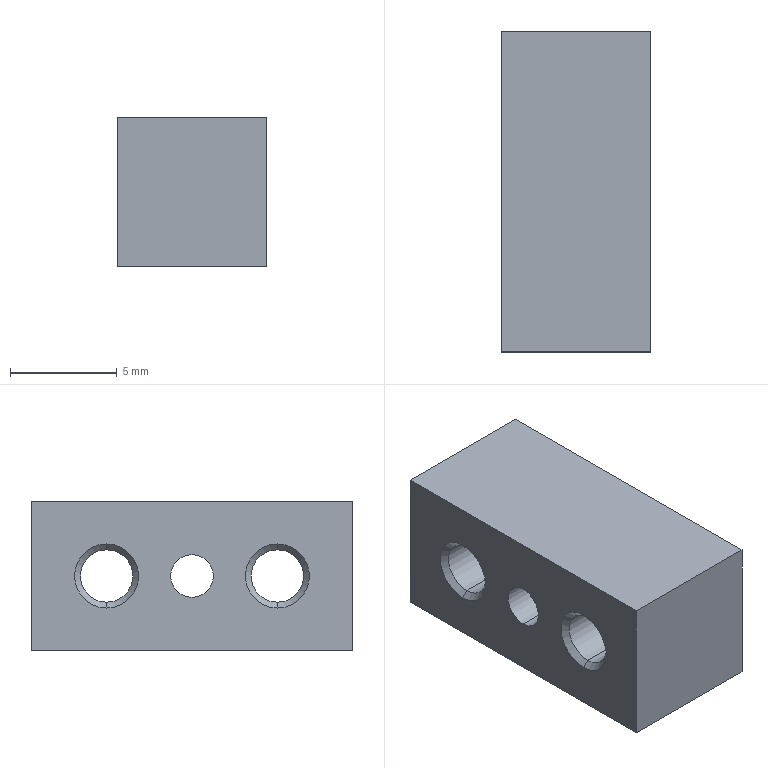Part | STEP file | 1 solid | 20 faces | box 7 x 15 x 7 mm | volume 645.309 mm3 | cone 8 | cylinder 6 | plane 6 | commonest cylinder face diameters 2.459 x4 2 x2
STEP:
#1=CARTESIAN_POINT('',(0.,0.,0.));
#2=DIRECTION('',(0.,0.,1.));
#3=DIRECTION('',(1.,0.,0.));
#4=AXIS2_PLACEMENT_3D('',#1,#2,#3);
#5=CARTESIAN_POINT('',(6.729,11.5,-1.23));
#6=VERTEX_POINT('',#5);
#7=CARTESIAN_POINT('',(7.,11.5,-1.5));
#8=VERTEX_POINT('',#7);
#9=CARTESIAN_POINT('',(7.,11.5,-1.5));
#10=DIRECTION('',(0.7071,0.,-0.7071));
#11=VECTOR('',#10,1.);
#12=LINE('',#9,#11);
#13=CARTESIAN_POINT('',(7.,11.5,0.));
#14=DIRECTION('',(1.,0.,0.));
#15=DIRECTION('',(0.,0.,-1.));
#16=AXIS2_PLACEMENT_3D('',#13,#14,#15);
#17=CONICAL_SURFACE('',#16,1.5,0.7854);
#18=CARTESIAN_POINT('',(6.283,0.));
#19=DIRECTION('',(0.,1.));
#20=VECTOR('',#19,1.);
#21=LINE('',#18,#20);
#22=(GEOMETRIC_REPRESENTATION_CONTEXT(2)PARAMETRIC_REPRESENTATION_CONTEXT()REPRESENTATION_CONTEXT('',''));
#23=DEFINITIONAL_REPRESENTATION('',(#21),#22);
#24=PCURVE('',#17,#23);
#25=CARTESIAN_POINT('',(7.,11.5,0.));
#26=DIRECTION('',(1.,0.,0.));
#27=DIRECTION('',(0.,0.,-1.));
#28=AXIS2_PLACEMENT_3D('',#25,#26,#27);
#29=CONICAL_SURFACE('',#28,1.5,0.7854);
#30=CARTESIAN_POINT('',(0.,0.));
#31=DIRECTION('',(0.,1.));
#32=VECTOR('',#31,1.);
#33=LINE('',#30,#32);
#34=(GEOMETRIC_REPRESENTATION_CONTEXT(2)PARAMETRIC_REPRESENTATION_CONTEXT()REPRESENTATION_CONTEXT('',''));
#35=DEFINITIONAL_REPRESENTATION('',(#33),#34);
#36=PCURVE('',#29,#35);
#37=SURFACE_CURVE('',#12,(#24,#36),.PCURVE_S1.);
#38=EDGE_CURVE('',#6,#8,#37,.T.);
#39=ORIENTED_EDGE('',*,*,#38,.T.);
#40=CARTESIAN_POINT('',(7.,11.5,1.5));
#41=VERTEX_POINT('',#40);
#42=CARTESIAN_POINT('',(7.,11.5,0.));
#43=DIRECTION('',(1.,0.,0.));
#44=DIRECTION('',(0.,0.,-1.));
#45=AXIS2_PLACEMENT_3D('',#42,#43,#44);
#46=CIRCLE('',#45,1.5);
#47=CARTESIAN_POINT('',(0.,0.));
#48=DIRECTION('',(1.,0.));
#49=VECTOR('',#48,1.);
#50=LINE('',#47,#49);
#51=(GEOMETRIC_REPRESENTATION_CONTEXT(2)PARAMETRIC_REPRESENTATION_CONTEXT()REPRESENTATION_CONTEXT('',''));
#52=DEFINITIONAL_REPRESENTATION('',(#50),#51);
#53=PCURVE('',#17,#52);
#54=CARTESIAN_POINT('',(7.,0.,3.5));
#55=DIRECTION('',(-1.,0.,0.));
#56=DIRECTION('',(0.,0.,1.));
#57=AXIS2_PLACEMENT_3D('',#54,#55,#56);
#58=PLANE('',#57);
#59=CARTESIAN_POINT('',(-5.,11.5));
#60=CARTESIAN_POINT('',(-5.,14.098));
#61=CARTESIAN_POINT('',(-2.75,12.799));
#62=CARTESIAN_POINT('',(-0.5,11.5));
#63=CARTESIAN_POINT('',(-2.75,10.201));
#64=CARTESIAN_POINT('',(-5.,8.902));
#65=CARTESIAN_POINT('',(-5.,11.5));
#66=(BOUNDED_CURVE()B_SPLINE_CURVE(2,(#59,#60,#61,#62,#63,#64,#65),.UNSPECIFIED.,.T.,.F.)B_SPLINE_CURVE_WITH_KNOTS((1,2,2,2,2,1),(-2.094,0.,2.094,4.189,6.283,8.378),.UNSPECIFIED.)CURVE()GEOMETRIC_REPRESENTATION_ITEM()RATIONAL_B_SPLINE_CURVE((1.,0.5,1.,0.5,1.,0.5,1.))REPRESENTATION_ITEM(''));
#67=(GEOMETRIC_REPRESENTATION_CONTEXT(2)PARAMETRIC_REPRESENTATION_CONTEXT()REPRESENTATION_CONTEXT('',''));
#68=DEFINITIONAL_REPRESENTATION('',(#66),#67);
#69=PCURVE('',#58,#68);
#70=SURFACE_CURVE('',#46,(#53,#69),.PCURVE_S1.);
#71=EDGE_CURVE('',#41,#8,#70,.T.);
#72=ORIENTED_EDGE('',*,*,#71,.F.);
#73=CARTESIAN_POINT('',(6.729,11.5,1.23));
#74=VERTEX_POINT('',#73);
#75=CARTESIAN_POINT('',(7.,11.5,1.5));
#76=DIRECTION('',(0.7071,0.,0.7071));
#77=VECTOR('',#76,1.);
#78=LINE('',#75,#77);
#79=CARTESIAN_POINT('',(3.142,0.));
#80=DIRECTION('',(0.,1.));
#81=VECTOR('',#80,1.);
#82=LINE('',#79,#81);
#83=(GEOMETRIC_REPRESENTATION_CONTEXT(2)PARAMETRIC_REPRESENTATION_CONTEXT()REPRESENTATION_CONTEXT('',''));
#84=DEFINITIONAL_REPRESENTATION('',(#82),#83);
#85=PCURVE('',#17,#84);
#86=CARTESIAN_POINT('',(3.142,0.));
#87=DIRECTION('',(0.,1.));
#88=VECTOR('',#87,1.);
#89=LINE('',#86,#88);
#90=(GEOMETRIC_REPRESENTATION_CONTEXT(2)PARAMETRIC_REPRESENTATION_CONTEXT()REPRESENTATION_CONTEXT('',''));
#91=DEFINITIONAL_REPRESENTATION('',(#89),#90);
#92=PCURVE('',#29,#91);
#93=SURFACE_CURVE('',#78,(#85,#92),.PCURVE_S1.);
#94=EDGE_CURVE('',#74,#41,#93,.T.);
#95=ORIENTED_EDGE('',*,*,#94,.F.);
#96=CARTESIAN_POINT('',(6.729,11.5,0.));
#97=DIRECTION('',(1.,0.,0.));
#98=DIRECTION('',(0.,0.,-1.));
#99=AXIS2_PLACEMENT_3D('',#96,#97,#98);
#100=CIRCLE('',#99,1.23);
#101=CARTESIAN_POINT('',(0.,-0.2705));
#102=DIRECTION('',(1.,0.));
#103=VECTOR('',#102,1.);
#104=LINE('',#101,#103);
#105=(GEOMETRIC_REPRESENTATION_CONTEXT(2)PARAMETRIC_REPRESENTATION_CONTEXT()REPRESENTATION_CONTEXT('',''));
#106=DEFINITIONAL_REPRESENTATION('',(#104),#105);
#107=PCURVE('',#17,#106);
#108=CARTESIAN_POINT('',(7.,11.5,0.));
#109=DIRECTION('',(1.,0.,0.));
#110=DIRECTION('',(0.,0.,-1.));
#111=AXIS2_PLACEMENT_3D('',#108,#109,#110);
#112=CYLINDRICAL_SURFACE('',#111,1.23);
#113=CARTESIAN_POINT('',(0.,-0.2705));
#114=DIRECTION('',(1.,0.));
#115=VECTOR('',#114,1.);
#116=LINE('',#113,#115);
#117=(GEOMETRIC_REPRESENTATION_CONTEXT(2)PARAMETRIC_REPRESENTATION_CONTEXT()REPRESENTATION_CONTEXT('',''));
#118=DEFINITIONAL_REPRESENTATION('',(#116),#117);
#119=PCURVE('',#112,#118);
#120=SURFACE_CURVE('',#100,(#107,#119),.PCURVE_S1.);
#121=EDGE_CURVE('',#74,#6,#120,.T.);
#122=ORIENTED_EDGE('',*,*,#121,.T.);
#123=EDGE_LOOP('',(#39,#72,#95,#122));
#124=FACE_BOUND('',#123,.F.);
#125=ADVANCED_FACE('',(#124),#17,.F.);
#126=CARTESIAN_POINT('',(0.2705,11.5,-1.23));
#127=VERTEX_POINT('',#126);
#128=CARTESIAN_POINT('',(7.,11.5,-1.23));
#129=DIRECTION('',(1.,0.,0.));
#130=VECTOR('',#129,1.);
#131=LINE('',#128,#130);
#132=CARTESIAN_POINT('',(6.283,0.));
#133=DIRECTION('',(0.,1.));
#134=VECTOR('',#133,1.);
#135=LINE('',#132,#134);
#136=(GEOMETRIC_REPRESENTATION_CONTEXT(2)PARAMETRIC_REPRESENTATION_CONTEXT()REPRESENTATION_CONTEXT('',''));
#137=DEFINITIONAL_REPRESENTATION('',(#135),#136);
#138=PCURVE('',#112,#137);
#139=CARTESIAN_POINT('',(7.,11.5,0.));
#140=DIRECTION('',(1.,0.,0.));
#141=DIRECTION('',(0.,0.,-1.));
#142=AXIS2_PLACEMENT_3D('',#139,#140,#141);
#143=CYLINDRICAL_SURFACE('',#142,1.23);
#144=CARTESIAN_POINT('',(0.,0.));
#145=DIRECTION('',(0.,1.));
#146=VECTOR('',#145,1.);
#147=LINE('',#144,#146);
#148=(GEOMETRIC_REPRESENTATION_CONTEXT(2)PARAMETRIC_REPRESENTATION_CONTEXT()REPRESENTATION_CONTEXT('',''));
#149=DEFINITIONAL_REPRESENTATION('',(#147),#148);
#150=PCURVE('',#143,#149);
#151=SURFACE_CURVE('',#131,(#138,#150),.PCURVE_S1.);
#152=EDGE_CURVE('',#127,#6,#151,.T.);
#153=ORIENTED_EDGE('',*,*,#152,.T.);
#154=ORIENTED_EDGE('',*,*,#121,.F.);
#155=CARTESIAN_POINT('',(0.2705,11.5,1.23));
#156=VERTEX_POINT('',#155);
#157=CARTESIAN_POINT('',(7.,11.5,1.23));
#158=DIRECTION('',(1.,0.,0.));
#159=VECTOR('',#158,1.);
#160=LINE('',#157,#159);
#161=CARTESIAN_POINT('',(3.142,0.));
#162=DIRECTION('',(0.,1.));
#163=VECTOR('',#162,1.);
#164=LINE('',#161,#163);
#165=(GEOMETRIC_REPRESENTATION_CONTEXT(2)PARAMETRIC_REPRESENTATION_CONTEXT()REPRESENTATION_CONTEXT('',''));
#166=DEFINITIONAL_REPRESENTATION('',(#164),#165);
#167=PCURVE('',#112,#166);
#168=CARTESIAN_POINT('',(3.142,0.));
#169=DIRECTION('',(0.,1.));
#170=VECTOR('',#169,1.);
#171=LINE('',#168,#170);
#172=(GEOMETRIC_REPRESENTATION_CONTEXT(2)PARAMETRIC_REPRESENTATION_CONTEXT()REPRESENTATION_CONTEXT('',''));
#173=DEFINITIONAL_REPRESENTATION('',(#171),#172);
#174=PCURVE('',#143,#173);
#175=SURFACE_CURVE('',#160,(#167,#174),.PCURVE_S1.);
#176=EDGE_CURVE('',#156,#74,#175,.T.);
#177=ORIENTED_EDGE('',*,*,#176,.F.);
#178=CARTESIAN_POINT('',(0.2705,11.5,0.));
#179=DIRECTION('',(1.,0.,0.));
#180=DIRECTION('',(0.,0.,-1.));
#181=AXIS2_PLACEMENT_3D('',#178,#179,#180);
#182=CIRCLE('',#181,1.23);
#183=CARTESIAN_POINT('',(0.,-6.729));
#184=DIRECTION('',(1.,0.));
#185=VECTOR('',#184,1.);
#186=LINE('',#183,#185);
#187=(GEOMETRIC_REPRESENTATION_CONTEXT(2)PARAMETRIC_REPRESENTATION_CONTEXT()REPRESENTATION_CONTEXT('',''));
#188=DEFINITIONAL_REPRESENTATION('',(#186),#187);
#189=PCURVE('',#112,#188);
#190=CARTESIAN_POINT('',(0.2705,11.5,0.));
#191=DIRECTION('',(-1.,0.,0.));
#192=DIRECTION('',(0.,0.,1.));
#193=AXIS2_PLACEMENT_3D('',#190,#191,#192);
#194=CONICAL_SURFACE('',#193,1.23,0.7854);
#195=CARTESIAN_POINT('',(9.425,0.));
#196=DIRECTION('',(-1.,0.));
#197=VECTOR('',#196,1.);
#198=LINE('',#195,#197);
#199=(GEOMETRIC_REPRESENTATION_CONTEXT(2)PARAMETRIC_REPRESENTATION_CONTEXT()REPRESENTATION_CONTEXT('',''));
#200=DEFINITIONAL_REPRESENTATION('',(#198),#199);
#201=PCURVE('',#194,#200);
#202=SURFACE_CURVE('',#182,(#189,#201),.PCURVE_S1.);
#203=EDGE_CURVE('',#156,#127,#202,.T.);
#204=ORIENTED_EDGE('',*,*,#203,.T.);
#205=EDGE_LOOP('',(#153,#154,#177,#204));
#206=FACE_BOUND('',#205,.F.);
#207=ADVANCED_FACE('',(#206),#112,.F.);
#208=CARTESIAN_POINT('',(0.,11.5,1.5));
#209=VERTEX_POINT('',#208);
#210=CARTESIAN_POINT('',(0.2705,11.5,1.23));
#211=DIRECTION('',(-0.7071,0.,0.7071));
#212=VECTOR('',#211,1.);
#213=LINE('',#210,#212);
#214=CARTESIAN_POINT('',(6.283,0.));
#215=DIRECTION('',(0.,1.));
#216=VECTOR('',#215,1.);
#217=LINE('',#214,#216);
#218=(GEOMETRIC_REPRESENTATION_CONTEXT(2)PARAMETRIC_REPRESENTATION_CONTEXT()REPRESENTATION_CONTEXT('',''));
#219=DEFINITIONAL_REPRESENTATION('',(#217),#218);
#220=PCURVE('',#194,#219);
#221=CARTESIAN_POINT('',(0.2705,11.5,0.));
#222=DIRECTION('',(-1.,0.,0.));
#223=DIRECTION('',(0.,0.,1.));
#224=AXIS2_PLACEMENT_3D('',#221,#222,#223);
#225=CONICAL_SURFACE('',#224,1.23,0.7854);
#226=CARTESIAN_POINT('',(0.,0.));
#227=DIRECTION('',(0.,1.));
#228=VECTOR('',#227,1.);
#229=LINE('',#226,#228);
#230=(GEOMETRIC_REPRESENTATION_CONTEXT(2)PARAMETRIC_REPRESENTATION_CONTEXT()REPRESENTATION_CONTEXT('',''));
#231=DEFINITIONAL_REPRESENTATION('',(#229),#230);
#232=PCURVE('',#225,#231);
#233=SURFACE_CURVE('',#213,(#220,#232),.PCURVE_S1.);
#234=EDGE_CURVE('',#156,#209,#233,.T.);
#235=ORIENTED_EDGE('',*,*,#234,.T.);
#236=CARTESIAN_POINT('',(0.,11.5,-1.5));
#237=VERTEX_POINT('',#236);
#238=CARTESIAN_POINT('',(0.,11.5,0.));
#239=DIRECTION('',(1.,0.,0.));
#240=DIRECTION('',(0.,0.,-1.));
#241=AXIS2_PLACEMENT_3D('',#238,#239,#240);
#242=CIRCLE('',#241,1.5);
#243=CARTESIAN_POINT('',(9.425,0.2705));
#244=DIRECTION('',(-1.,0.));
#245=VECTOR('',#244,1.);
#246=LINE('',#243,#245);
#247=(GEOMETRIC_REPRESENTATION_CONTEXT(2)PARAMETRIC_REPRESENTATION_CONTEXT()REPRESENTATION_CONTEXT('',''));
#248=DEFINITIONAL_REPRESENTATION('',(#246),#247);
#249=PCURVE('',#194,#248);
#250=CARTESIAN_POINT('',(0.,15.,3.5));
#251=DIRECTION('',(1.,0.,0.));
#252=DIRECTION('',(0.,0.,-1.));
#253=AXIS2_PLACEMENT_3D('',#250,#251,#252);
#254=PLANE('',#253);
#255=CARTESIAN_POINT('',(3.5,-3.5));
#256=DIRECTION('',(1.,0.));
#257=AXIS2_PLACEMENT_2D('',#255,#256);
#258=CIRCLE('',#257,1.5);
#259=(GEOMETRIC_REPRESENTATION_CONTEXT(2)PARAMETRIC_REPRESENTATION_CONTEXT()REPRESENTATION_CONTEXT('',''));
#260=DEFINITIONAL_REPRESENTATION('',(#258),#259);
#261=PCURVE('',#254,#260);
#262=SURFACE_CURVE('',#242,(#249,#261),.PCURVE_S1.);
#263=EDGE_CURVE('',#209,#237,#262,.T.);
#264=ORIENTED_EDGE('',*,*,#263,.T.);
#265=CARTESIAN_POINT('',(0.2705,11.5,-1.23));
#266=DIRECTION('',(-0.7071,0.,-0.7071));
#267=VECTOR('',#266,1.);
#268=LINE('',#265,#267);
#269=CARTESIAN_POINT('',(3.142,0.));
#270=DIRECTION('',(0.,1.));
#271=VECTOR('',#270,1.);
#272=LINE('',#269,#271);
#273=(GEOMETRIC_REPRESENTATION_CONTEXT(2)PARAMETRIC_REPRESENTATION_CONTEXT()REPRESENTATION_CONTEXT('',''));
#274=DEFINITIONAL_REPRESENTATION('',(#272),#273);
#275=PCURVE('',#194,#274);
#276=CARTESIAN_POINT('',(3.142,0.));
#277=DIRECTION('',(0.,1.));
#278=VECTOR('',#277,1.);
#279=LINE('',#276,#278);
#280=(GEOMETRIC_REPRESENTATION_CONTEXT(2)PARAMETRIC_REPRESENTATION_CONTEXT()REPRESENTATION_CONTEXT('',''));
#281=DEFINITIONAL_REPRESENTATION('',(#279),#280);
#282=PCURVE('',#225,#281);
#283=SURFACE_CURVE('',#268,(#275,#282),.PCURVE_S1.);
#284=EDGE_CURVE('',#127,#237,#283,.T.);
#285=ORIENTED_EDGE('',*,*,#284,.F.);
#286=ORIENTED_EDGE('',*,*,#203,.F.);
#287=EDGE_LOOP('',(#235,#264,#285,#286));
#288=FACE_BOUND('',#287,.F.);
#289=ADVANCED_FACE('',(#288),#194,.F.);
#290=CARTESIAN_POINT('',(6.729,3.5,-1.23));
#291=VERTEX_POINT('',#290);
#292=CARTESIAN_POINT('',(7.,3.5,-1.5));
#293=VERTEX_POINT('',#292);
#294=CARTESIAN_POINT('',(7.,3.5,-1.5));
#295=DIRECTION('',(0.7071,0.,-0.7071));
#296=VECTOR('',#295,1.);
#297=LINE('',#294,#296);
#298=CARTESIAN_POINT('',(7.,3.5,0.));
#299=DIRECTION('',(1.,0.,0.));
#300=DIRECTION('',(0.,0.,-1.));
#301=AXIS2_PLACEMENT_3D('',#298,#299,#300);
#302=CONICAL_SURFACE('',#301,1.5,0.7854);
#303=CARTESIAN_POINT('',(6.283,0.));
#304=DIRECTION('',(0.,1.));
#305=VECTOR('',#304,1.);
#306=LINE('',#303,#305);
#307=(GEOMETRIC_REPRESENTATION_CONTEXT(2)PARAMETRIC_REPRESENTATION_CONTEXT()REPRESENTATION_CONTEXT('',''));
#308=DEFINITIONAL_REPRESENTATION('',(#306),#307);
#309=PCURVE('',#302,#308);
#310=CARTESIAN_POINT('',(7.,3.5,0.));
#311=DIRECTION('',(1.,0.,0.));
#312=DIRECTION('',(0.,0.,-1.));
#313=AXIS2_PLACEMENT_3D('',#310,#311,#312);
#314=CONICAL_SURFACE('',#313,1.5,0.7854);
#315=CARTESIAN_POINT('',(0.,0.));
#316=DIRECTION('',(0.,1.));
#317=VECTOR('',#316,1.);
#318=LINE('',#315,#317);
#319=(GEOMETRIC_REPRESENTATION_CONTEXT(2)PARAMETRIC_REPRESENTATION_CONTEXT()REPRESENTATION_CONTEXT('',''));
#320=DEFINITIONAL_REPRESENTATION('',(#318),#319);
#321=PCURVE('',#314,#320);
#322=SURFACE_CURVE('',#297,(#309,#321),.PCURVE_S1.);
#323=EDGE_CURVE('',#291,#293,#322,.T.);
#324=ORIENTED_EDGE('',*,*,#323,.T.);
#325=CARTESIAN_POINT('',(7.,3.5,1.5));
#326=VERTEX_POINT('',#325);
#327=CARTESIAN_POINT('',(7.,3.5,0.));
#328=DIRECTION('',(1.,0.,0.));
#329=DIRECTION('',(0.,0.,-1.));
#330=AXIS2_PLACEMENT_3D('',#327,#328,#329);
#331=CIRCLE('',#330,1.5);
#332=CARTESIAN_POINT('',(0.,0.));
#333=DIRECTION('',(1.,0.));
#334=VECTOR('',#333,1.);
#335=LINE('',#332,#334);
#336=(GEOMETRIC_REPRESENTATION_CONTEXT(2)PARAMETRIC_REPRESENTATION_CONTEXT()REPRESENTATION_CONTEXT('',''));
#337=DEFINITIONAL_REPRESENTATION('',(#335),#336);
#338=PCURVE('',#302,#337);
#339=CARTESIAN_POINT('',(-5.,3.5));
#340=CARTESIAN_POINT('',(-5.,6.098));
#341=CARTESIAN_POINT('',(-2.75,4.799));
#342=CARTESIAN_POINT('',(-0.5,3.5));
#343=CARTESIAN_POINT('',(-2.75,2.201));
#344=CARTESIAN_POINT('',(-5.,0.9019));
#345=CARTESIAN_POINT('',(-5.,3.5));
#346=(BOUNDED_CURVE()B_SPLINE_CURVE(2,(#339,#340,#341,#342,#343,#344,#345),.UNSPECIFIED.,.T.,.F.)B_SPLINE_CURVE_WITH_KNOTS((1,2,2,2,2,1),(-2.094,0.,2.094,4.189,6.283,8.378),.UNSPECIFIED.)CURVE()GEOMETRIC_REPRESENTATION_ITEM()RATIONAL_B_SPLINE_CURVE((1.,0.5,1.,0.5,1.,0.5,1.))REPRESENTATION_ITEM(''));
#347=(GEOMETRIC_REPRESENTATION_CONTEXT(2)PARAMETRIC_REPRESENTATION_CONTEXT()REPRESENTATION_CONTEXT('',''));
#348=DEFINITIONAL_REPRESENTATION('',(#346),#347);
#349=PCURVE('',#58,#348);
#350=SURFACE_CURVE('',#331,(#338,#349),.PCURVE_S1.);
#351=EDGE_CURVE('',#326,#293,#350,.T.);
#352=ORIENTED_EDGE('',*,*,#351,.F.);
#353=CARTESIAN_POINT('',(6.729,3.5,1.23));
#354=VERTEX_POINT('',#353);
#355=CARTESIAN_POINT('',(7.,3.5,1.5));
#356=DIRECTION('',(0.7071,0.,0.7071));
#357=VECTOR('',#356,1.);
#358=LINE('',#355,#357);
#359=CARTESIAN_POINT('',(3.142,0.));
#360=DIRECTION('',(0.,1.));
#361=VECTOR('',#360,1.);
#362=LINE('',#359,#361);
#363=(GEOMETRIC_REPRESENTATION_CONTEXT(2)PARAMETRIC_REPRESENTATION_CONTEXT()REPRESENTATION_CONTEXT('',''));
#364=DEFINITIONAL_REPRESENTATION('',(#362),#363);
#365=PCURVE('',#302,#364);
#366=CARTESIAN_POINT('',(3.142,0.));
#367=DIRECTION('',(0.,1.));
#368=VECTOR('',#367,1.);
#369=LINE('',#366,#368);
#370=(GEOMETRIC_REPRESENTATION_CONTEXT(2)PARAMETRIC_REPRESENTATION_CONTEXT()REPRESENTATION_CONTEXT('',''));
#371=DEFINITIONAL_REPRESENTATION('',(#369),#370);
#372=PCURVE('',#314,#371);
#373=SURFACE_CURVE('',#358,(#365,#372),.PCURVE_S1.);
#374=EDGE_CURVE('',#354,#326,#373,.T.);
#375=ORIENTED_EDGE('',*,*,#374,.F.);
#376=CARTESIAN_POINT('',(6.729,3.5,0.));
#377=DIRECTION('',(1.,0.,0.));
#378=DIRECTION('',(0.,0.,-1.));
#379=AXIS2_PLACEMENT_3D('',#376,#377,#378);
#380=CIRCLE('',#379,1.23);
#381=CARTESIAN_POINT('',(0.,-0.2705));
#382=DIRECTION('',(1.,0.));
#383=VECTOR('',#382,1.);
#384=LINE('',#381,#383);
#385=(GEOMETRIC_REPRESENTATION_CONTEXT(2)PARAMETRIC_REPRESENTATION_CONTEXT()REPRESENTATION_CONTEXT('',''));
#386=DEFINITIONAL_REPRESENTATION('',(#384),#385);
#387=PCURVE('',#302,#386);
#388=CARTESIAN_POINT('',(7.,3.5,0.));
#389=DIRECTION('',(1.,0.,0.));
#390=DIRECTION('',(0.,0.,-1.));
#391=AXIS2_PLACEMENT_3D('',#388,#389,#390);
#392=CYLINDRICAL_SURFACE('',#391,1.23);
#393=CARTESIAN_POINT('',(0.,-0.2705));
#394=DIRECTION('',(1.,0.));
#395=VECTOR('',#394,1.);
#396=LINE('',#393,#395);
#397=(GEOMETRIC_REPRESENTATION_CONTEXT(2)PARAMETRIC_REPRESENTATION_CONTEXT()REPRESENTATION_CONTEXT('',''));
#398=DEFINITIONAL_REPRESENTATION('',(#396),#397);
#399=PCURVE('',#392,#398);
#400=SURFACE_CURVE('',#380,(#387,#399),.PCURVE_S1.);
#401=EDGE_CURVE('',#354,#291,#400,.T.);
#402=ORIENTED_EDGE('',*,*,#401,.T.);
#403=EDGE_LOOP('',(#324,#352,#375,#402));
#404=FACE_BOUND('',#403,.F.);
#405=ADVANCED_FACE('',(#404),#302,.F.);
#406=CARTESIAN_POINT('',(0.2705,3.5,-1.23));
#407=VERTEX_POINT('',#406);
#408=CARTESIAN_POINT('',(7.,3.5,-1.23));
#409=DIRECTION('',(1.,0.,0.));
#410=VECTOR('',#409,1.);
#411=LINE('',#408,#410);
#412=CARTESIAN_POINT('',(6.283,0.));
#413=DIRECTION('',(0.,1.));
#414=VECTOR('',#413,1.);
#415=LINE('',#412,#414);
#416=(GEOMETRIC_REPRESENTATION_CONTEXT(2)PARAMETRIC_REPRESENTATION_CONTEXT()REPRESENTATION_CONTEXT('',''));
#417=DEFINITIONAL_REPRESENTATION('',(#415),#416);
#418=PCURVE('',#392,#417);
#419=CARTESIAN_POINT('',(7.,3.5,0.));
#420=DIRECTION('',(1.,0.,0.));
#421=DIRECTION('',(0.,0.,-1.));
#422=AXIS2_PLACEMENT_3D('',#419,#420,#421);
#423=CYLINDRICAL_SURFACE('',#422,1.23);
#424=CARTESIAN_POINT('',(0.,0.));
#425=DIRECTION('',(0.,1.));
#426=VECTOR('',#425,1.);
#427=LINE('',#424,#426);
#428=(GEOMETRIC_REPRESENTATION_CONTEXT(2)PARAMETRIC_REPRESENTATION_CONTEXT()REPRESENTATION_CONTEXT('',''));
#429=DEFINITIONAL_REPRESENTATION('',(#427),#428);
#430=PCURVE('',#423,#429);
#431=SURFACE_CURVE('',#411,(#418,#430),.PCURVE_S1.);
#432=EDGE_CURVE('',#407,#291,#431,.T.);
#433=ORIENTED_EDGE('',*,*,#432,.T.);
#434=ORIENTED_EDGE('',*,*,#401,.F.);
#435=CARTESIAN_POINT('',(0.2705,3.5,1.23));
#436=VERTEX_POINT('',#435);
#437=CARTESIAN_POINT('',(7.,3.5,1.23));
#438=DIRECTION('',(1.,0.,0.));
#439=VECTOR('',#438,1.);
#440=LINE('',#437,#439);
#441=CARTESIAN_POINT('',(3.142,0.));
#442=DIRECTION('',(0.,1.));
#443=VECTOR('',#442,1.);
#444=LINE('',#441,#443);
#445=(GEOMETRIC_REPRESENTATION_CONTEXT(2)PARAMETRIC_REPRESENTATION_CONTEXT()REPRESENTATION_CONTEXT('',''));
#446=DEFINITIONAL_REPRESENTATION('',(#444),#445);
#447=PCURVE('',#392,#446);
#448=CARTESIAN_POINT('',(3.142,0.));
#449=DIRECTION('',(0.,1.));
#450=VECTOR('',#449,1.);
#451=LINE('',#448,#450);
#452=(GEOMETRIC_REPRESENTATION_CONTEXT(2)PARAMETRIC_REPRESENTATION_CONTEXT()REPRESENTATION_CONTEXT('',''));
#453=DEFINITIONAL_REPRESENTATION('',(#451),#452);
#454=PCURVE('',#423,#453);
#455=SURFACE_CURVE('',#440,(#447,#454),.PCURVE_S1.);
#456=EDGE_CURVE('',#436,#354,#455,.T.);
#457=ORIENTED_EDGE('',*,*,#456,.F.);
#458=CARTESIAN_POINT('',(0.2705,3.5,0.));
#459=DIRECTION('',(1.,0.,0.));
#460=DIRECTION('',(0.,0.,-1.));
#461=AXIS2_PLACEMENT_3D('',#458,#459,#460);
#462=CIRCLE('',#461,1.23);
#463=CARTESIAN_POINT('',(0.,-6.729));
#464=DIRECTION('',(1.,0.));
#465=VECTOR('',#464,1.);
#466=LINE('',#463,#465);
#467=(GEOMETRIC_REPRESENTATION_CONTEXT(2)PARAMETRIC_REPRESENTATION_CONTEXT()REPRESENTATION_CONTEXT('',''));
#468=DEFINITIONAL_REPRESENTATION('',(#466),#467);
#469=PCURVE('',#392,#468);
#470=CARTESIAN_POINT('',(0.2705,3.5,0.));
#471=DIRECTION('',(-1.,0.,0.));
#472=DIRECTION('',(0.,0.,1.));
#473=AXIS2_PLACEMENT_3D('',#470,#471,#472);
#474=CONICAL_SURFACE('',#473,1.23,0.7854);
#475=CARTESIAN_POINT('',(9.425,0.));
#476=DIRECTION('',(-1.,0.));
#477=VECTOR('',#476,1.);
#478=LINE('',#475,#477);
#479=(GEOMETRIC_REPRESENTATION_CONTEXT(2)PARAMETRIC_REPRESENTATION_CONTEXT()REPRESENTATION_CONTEXT('',''));
#480=DEFINITIONAL_REPRESENTATION('',(#478),#479);
#481=PCURVE('',#474,#480);
#482=SURFACE_CURVE('',#462,(#469,#481),.PCURVE_S1.);
#483=EDGE_CURVE('',#436,#407,#482,.T.);
#484=ORIENTED_EDGE('',*,*,#483,.T.);
#485=EDGE_LOOP('',(#433,#434,#457,#484));
#486=FACE_BOUND('',#485,.F.);
#487=ADVANCED_FACE('',(#486),#392,.F.);
#488=CARTESIAN_POINT('',(0.,3.5,1.5));
#489=VERTEX_POINT('',#488);
#490=CARTESIAN_POINT('',(0.2705,3.5,1.23));
#491=DIRECTION('',(-0.7071,0.,0.7071));
#492=VECTOR('',#491,1.);
#493=LINE('',#490,#492);
#494=CARTESIAN_POINT('',(6.283,0.));
#495=DIRECTION('',(0.,1.));
#496=VECTOR('',#495,1.);
#497=LINE('',#494,#496);
#498=(GEOMETRIC_REPRESENTATION_CONTEXT(2)PARAMETRIC_REPRESENTATION_CONTEXT()REPRESENTATION_CONTEXT('',''));
#499=DEFINITIONAL_REPRESENTATION('',(#497),#498);
#500=PCURVE('',#474,#499);
#501=CARTESIAN_POINT('',(0.2705,3.5,0.));
#502=DIRECTION('',(-1.,0.,0.));
#503=DIRECTION('',(0.,0.,1.));
#504=AXIS2_PLACEMENT_3D('',#501,#502,#503);
#505=CONICAL_SURFACE('',#504,1.23,0.7854);
#506=CARTESIAN_POINT('',(0.,0.));
#507=DIRECTION('',(0.,1.));
#508=VECTOR('',#507,1.);
#509=LINE('',#506,#508);
#510=(GEOMETRIC_REPRESENTATION_CONTEXT(2)PARAMETRIC_REPRESENTATION_CONTEXT()REPRESENTATION_CONTEXT('',''));
#511=DEFINITIONAL_REPRESENTATION('',(#509),#510);
#512=PCURVE('',#505,#511);
#513=SURFACE_CURVE('',#493,(#500,#512),.PCURVE_S1.);
#514=EDGE_CURVE('',#436,#489,#513,.T.);
#515=ORIENTED_EDGE('',*,*,#514,.T.);
#516=CARTESIAN_POINT('',(0.,3.5,-1.5));
#517=VERTEX_POINT('',#516);
#518=CARTESIAN_POINT('',(0.,3.5,0.));
#519=DIRECTION('',(1.,0.,0.));
#520=DIRECTION('',(0.,0.,-1.));
#521=AXIS2_PLACEMENT_3D('',#518,#519,#520);
#522=CIRCLE('',#521,1.5);
#523=CARTESIAN_POINT('',(9.425,0.2705));
#524=DIRECTION('',(-1.,0.));
#525=VECTOR('',#524,1.);
#526=LINE('',#523,#525);
#527=(GEOMETRIC_REPRESENTATION_CONTEXT(2)PARAMETRIC_REPRESENTATION_CONTEXT()REPRESENTATION_CONTEXT('',''));
#528=DEFINITIONAL_REPRESENTATION('',(#526),#527);
#529=PCURVE('',#474,#528);
#530=CARTESIAN_POINT('',(3.5,-11.5));
#531=DIRECTION('',(1.,0.));
#532=AXIS2_PLACEMENT_2D('',#530,#531);
#533=CIRCLE('',#532,1.5);
#534=(GEOMETRIC_REPRESENTATION_CONTEXT(2)PARAMETRIC_REPRESENTATION_CONTEXT()REPRESENTATION_CONTEXT('',''));
#535=DEFINITIONAL_REPRESENTATION('',(#533),#534);
#536=PCURVE('',#254,#535);
#537=SURFACE_CURVE('',#522,(#529,#536),.PCURVE_S1.);
#538=EDGE_CURVE('',#489,#517,#537,.T.);
#539=ORIENTED_EDGE('',*,*,#538,.T.);
#540=CARTESIAN_POINT('',(0.2705,3.5,-1.23));
#541=DIRECTION('',(-0.7071,0.,-0.7071));
#542=VECTOR('',#541,1.);
#543=LINE('',#540,#542);
#544=CARTESIAN_POINT('',(3.142,0.));
#545=DIRECTION('',(0.,1.));
#546=VECTOR('',#545,1.);
#547=LINE('',#544,#546);
#548=(GEOMETRIC_REPRESENTATION_CONTEXT(2)PARAMETRIC_REPRESENTATION_CONTEXT()REPRESENTATION_CONTEXT('',''));
#549=DEFINITIONAL_REPRESENTATION('',(#547),#548);
#550=PCURVE('',#474,#549);
#551=CARTESIAN_POINT('',(3.142,0.));
#552=DIRECTION('',(0.,1.));
#553=VECTOR('',#552,1.);
#554=LINE('',#551,#553);
#555=(GEOMETRIC_REPRESENTATION_CONTEXT(2)PARAMETRIC_REPRESENTATION_CONTEXT()REPRESENTATION_CONTEXT('',''));
#556=DEFINITIONAL_REPRESENTATION('',(#554),#555);
#557=PCURVE('',#505,#556);
#558=SURFACE_CURVE('',#543,(#550,#557),.PCURVE_S1.);
#559=EDGE_CURVE('',#407,#517,#558,.T.);
#560=ORIENTED_EDGE('',*,*,#559,.F.);
#561=ORIENTED_EDGE('',*,*,#483,.F.);
#562=EDGE_LOOP('',(#515,#539,#560,#561));
#563=FACE_BOUND('',#562,.F.);
#564=ADVANCED_FACE('',(#563),#474,.F.);
#565=CARTESIAN_POINT('',(7.,7.5,1.));
#566=VERTEX_POINT('',#565);
#567=CARTESIAN_POINT('',(0.,7.5,1.));
#568=VERTEX_POINT('',#567);
#569=CARTESIAN_POINT('',(0.,7.5,1.));
#570=DIRECTION('',(-1.,0.,0.));
#571=VECTOR('',#570,1.);
#572=LINE('',#569,#571);
#573=CARTESIAN_POINT('',(0.,7.5,0.));
#574=DIRECTION('',(-1.,0.,0.));
#575=DIRECTION('',(0.,0.,1.));
#576=AXIS2_PLACEMENT_3D('',#573,#574,#575);
#577=CYLINDRICAL_SURFACE('',#576,1.);
#578=CARTESIAN_POINT('',(6.283,0.));
#579=DIRECTION('',(0.,1.));
#580=VECTOR('',#579,1.);
#581=LINE('',#578,#580);
#582=(GEOMETRIC_REPRESENTATION_CONTEXT(2)PARAMETRIC_REPRESENTATION_CONTEXT()REPRESENTATION_CONTEXT('',''));
#583=DEFINITIONAL_REPRESENTATION('',(#581),#582);
#584=PCURVE('',#577,#583);
#585=CARTESIAN_POINT('',(0.,7.5,0.));
#586=DIRECTION('',(-1.,0.,0.));
#587=DIRECTION('',(0.,0.,1.));
#588=AXIS2_PLACEMENT_3D('',#585,#586,#587);
#589=CYLINDRICAL_SURFACE('',#588,1.);
#590=CARTESIAN_POINT('',(0.,0.));
#591=DIRECTION('',(0.,1.));
#592=VECTOR('',#591,1.);
#593=LINE('',#590,#592);
#594=(GEOMETRIC_REPRESENTATION_CONTEXT(2)PARAMETRIC_REPRESENTATION_CONTEXT()REPRESENTATION_CONTEXT('',''));
#595=DEFINITIONAL_REPRESENTATION('',(#593),#594);
#596=PCURVE('',#589,#595);
#597=SURFACE_CURVE('',#572,(#584,#596),.PCURVE_S1.);
#598=EDGE_CURVE('',#566,#568,#597,.T.);
#599=ORIENTED_EDGE('',*,*,#598,.T.);
#600=CARTESIAN_POINT('',(0.,7.5,-1.));
#601=VERTEX_POINT('',#600);
#602=CARTESIAN_POINT('',(0.,7.5,0.));
#603=DIRECTION('',(-1.,0.,0.));
#604=DIRECTION('',(0.,0.,1.));
#605=AXIS2_PLACEMENT_3D('',#602,#603,#604);
#606=CIRCLE('',#605,1.);
#607=CARTESIAN_POINT('',(0.,0.));
#608=DIRECTION('',(1.,0.));
#609=VECTOR('',#608,1.);
#610=LINE('',#607,#609);
#611=(GEOMETRIC_REPRESENTATION_CONTEXT(2)PARAMETRIC_REPRESENTATION_CONTEXT()REPRESENTATION_CONTEXT('',''));
#612=DEFINITIONAL_REPRESENTATION('',(#610),#611);
#613=PCURVE('',#577,#612);
#614=CARTESIAN_POINT('',(2.5,-7.5));
#615=CARTESIAN_POINT('',(2.5,-5.768));
#616=CARTESIAN_POINT('',(4.,-6.634));
#617=CARTESIAN_POINT('',(5.5,-7.5));
#618=CARTESIAN_POINT('',(4.,-8.366));
#619=CARTESIAN_POINT('',(2.5,-9.232));
#620=CARTESIAN_POINT('',(2.5,-7.5));
#621=(BOUNDED_CURVE()B_SPLINE_CURVE(2,(#614,#615,#616,#617,#618,#619,#620),.UNSPECIFIED.,.T.,.F.)B_SPLINE_CURVE_WITH_KNOTS((1,2,2,2,2,1),(-2.094,0.,2.094,4.189,6.283,8.378),.UNSPECIFIED.)CURVE()GEOMETRIC_REPRESENTATION_ITEM()RATIONAL_B_SPLINE_CURVE((1.,0.5,1.,0.5,1.,0.5,1.))REPRESENTATION_ITEM(''));
#622=(GEOMETRIC_REPRESENTATION_CONTEXT(2)PARAMETRIC_REPRESENTATION_CONTEXT()REPRESENTATION_CONTEXT('',''));
#623=DEFINITIONAL_REPRESENTATION('',(#621),#622);
#624=PCURVE('',#254,#623);
#625=SURFACE_CURVE('',#606,(#613,#624),.PCURVE_S1.);
#626=EDGE_CURVE('',#601,#568,#625,.T.);
#627=ORIENTED_EDGE('',*,*,#626,.F.);
#628=CARTESIAN_POINT('',(7.,7.5,-1.));
#629=VERTEX_POINT('',#628);
#630=CARTESIAN_POINT('',(0.,7.5,-1.));
#631=DIRECTION('',(-1.,0.,0.));
#632=VECTOR('',#631,1.);
#633=LINE('',#630,#632);
#634=CARTESIAN_POINT('',(3.142,0.));
#635=DIRECTION('',(0.,1.));
#636=VECTOR('',#635,1.);
#637=LINE('',#634,#636);
#638=(GEOMETRIC_REPRESENTATION_CONTEXT(2)PARAMETRIC_REPRESENTATION_CONTEXT()REPRESENTATION_CONTEXT('',''));
#639=DEFINITIONAL_REPRESENTATION('',(#637),#638);
#640=PCURVE('',#577,#639);
#641=CARTESIAN_POINT('',(3.142,0.));
#642=DIRECTION('',(0.,1.));
#643=VECTOR('',#642,1.);
#644=LINE('',#641,#643);
#645=(GEOMETRIC_REPRESENTATION_CONTEXT(2)PARAMETRIC_REPRESENTATION_CONTEXT()REPRESENTATION_CONTEXT('',''));
#646=DEFINITIONAL_REPRESENTATION('',(#644),#645);
#647=PCURVE('',#589,#646);
#648=SURFACE_CURVE('',#633,(#640,#647),.PCURVE_S1.);
#649=EDGE_CURVE('',#629,#601,#648,.T.);
#650=ORIENTED_EDGE('',*,*,#649,.F.);
#651=CARTESIAN_POINT('',(7.,7.5,0.));
#652=DIRECTION('',(-1.,0.,0.));
#653=DIRECTION('',(0.,0.,1.));
#654=AXIS2_PLACEMENT_3D('',#651,#652,#653);
#655=CIRCLE('',#654,1.);
#656=CARTESIAN_POINT('',(0.,-7.));
#657=DIRECTION('',(1.,0.));
#658=VECTOR('',#657,1.);
#659=LINE('',#656,#658);
#660=(GEOMETRIC_REPRESENTATION_CONTEXT(2)PARAMETRIC_REPRESENTATION_CONTEXT()REPRESENTATION_CONTEXT('',''));
#661=DEFINITIONAL_REPRESENTATION('',(#659),#660);
#662=PCURVE('',#577,#661);
#663=CARTESIAN_POINT('',(-3.5,7.5));
#664=DIRECTION('',(1.,0.));
#665=AXIS2_PLACEMENT_2D('',#663,#664);
#666=CIRCLE('',#665,1.);
#667=(GEOMETRIC_REPRESENTATION_CONTEXT(2)PARAMETRIC_REPRESENTATION_CONTEXT()REPRESENTATION_CONTEXT('',''));
#668=DEFINITIONAL_REPRESENTATION('',(#666),#667);
#669=PCURVE('',#58,#668);
#670=SURFACE_CURVE('',#655,(#662,#669),.PCURVE_S1.);
#671=EDGE_CURVE('',#629,#566,#670,.T.);
#672=ORIENTED_EDGE('',*,*,#671,.T.);
#673=EDGE_LOOP('',(#599,#627,#650,#672));
#674=FACE_BOUND('',#673,.F.);
#675=ADVANCED_FACE('',(#674),#577,.F.);
#676=CARTESIAN_POINT('',(7.,15.,3.5));
#677=VERTEX_POINT('',#676);
#678=CARTESIAN_POINT('',(7.,15.,-3.5));
#679=VERTEX_POINT('',#678);
#680=CARTESIAN_POINT('',(7.,15.,3.5));
#681=DIRECTION('',(0.,0.,-1.));
#682=VECTOR('',#681,1.);
#683=LINE('',#680,#682);
#684=CARTESIAN_POINT('',(7.,15.,3.5));
#685=DIRECTION('',(0.,-1.,0.));
#686=DIRECTION('',(0.,0.,-1.));
#687=AXIS2_PLACEMENT_3D('',#684,#685,#686);
#688=PLANE('',#687);
#689=CARTESIAN_POINT('',(0.,0.));
#690=DIRECTION('',(1.,0.));
#691=VECTOR('',#690,1.);
#692=LINE('',#689,#691);
#693=(GEOMETRIC_REPRESENTATION_CONTEXT(2)PARAMETRIC_REPRESENTATION_CONTEXT()REPRESENTATION_CONTEXT('',''));
#694=DEFINITIONAL_REPRESENTATION('',(#692),#693);
#695=PCURVE('',#688,#694);
#696=CARTESIAN_POINT('',(0.,15.));
#697=DIRECTION('',(-1.,0.));
#698=VECTOR('',#697,1.);
#699=LINE('',#696,#698);
#700=(GEOMETRIC_REPRESENTATION_CONTEXT(2)PARAMETRIC_REPRESENTATION_CONTEXT()REPRESENTATION_CONTEXT('',''));
#701=DEFINITIONAL_REPRESENTATION('',(#699),#700);
#702=PCURVE('',#58,#701);
#703=SURFACE_CURVE('',#683,(#695,#702),.PCURVE_S1.);
#704=EDGE_CURVE('',#677,#679,#703,.T.);
#705=ORIENTED_EDGE('',*,*,#704,.T.);
#706=CARTESIAN_POINT('',(0.,15.,-3.5));
#707=VERTEX_POINT('',#706);
#708=CARTESIAN_POINT('',(7.,15.,-3.5));
#709=DIRECTION('',(-1.,0.,0.));
#710=VECTOR('',#709,1.);
#711=LINE('',#708,#710);
#712=CARTESIAN_POINT('',(7.,0.));
#713=DIRECTION('',(0.,-1.));
#714=VECTOR('',#713,1.);
#715=LINE('',#712,#714);
#716=(GEOMETRIC_REPRESENTATION_CONTEXT(2)PARAMETRIC_REPRESENTATION_CONTEXT()REPRESENTATION_CONTEXT('',''));
#717=DEFINITIONAL_REPRESENTATION('',(#715),#716);
#718=PCURVE('',#688,#717);
#719=CARTESIAN_POINT('',(0.,15.,-3.5));
#720=DIRECTION('',(0.,0.,1.));
#721=DIRECTION('',(1.,0.,0.));
#722=AXIS2_PLACEMENT_3D('',#719,#720,#721);
#723=PLANE('',#722);
#724=CARTESIAN_POINT('',(7.,0.));
#725=DIRECTION('',(-1.,0.));
#726=VECTOR('',#725,1.);
#727=LINE('',#724,#726);
#728=(GEOMETRIC_REPRESENTATION_CONTEXT(2)PARAMETRIC_REPRESENTATION_CONTEXT()REPRESENTATION_CONTEXT('',''));
#729=DEFINITIONAL_REPRESENTATION('',(#727),#728);
#730=PCURVE('',#723,#729);
#731=SURFACE_CURVE('',#711,(#718,#730),.PCURVE_S1.);
#732=EDGE_CURVE('',#679,#707,#731,.T.);
#733=ORIENTED_EDGE('',*,*,#732,.T.);
#734=CARTESIAN_POINT('',(0.,15.,3.5));
#735=VERTEX_POINT('',#734);
#736=CARTESIAN_POINT('',(0.,15.,3.5));
#737=DIRECTION('',(0.,0.,-1.));
#738=VECTOR('',#737,1.);
#739=LINE('',#736,#738);
#740=CARTESIAN_POINT('',(0.,-7.));
#741=DIRECTION('',(1.,0.));
#742=VECTOR('',#741,1.);
#743=LINE('',#740,#742);
#744=(GEOMETRIC_REPRESENTATION_CONTEXT(2)PARAMETRIC_REPRESENTATION_CONTEXT()REPRESENTATION_CONTEXT('',''));
#745=DEFINITIONAL_REPRESENTATION('',(#743),#744);
#746=PCURVE('',#688,#745);
#747=CARTESIAN_POINT('',(0.,0.));
#748=DIRECTION('',(1.,0.));
#749=VECTOR('',#748,1.);
#750=LINE('',#747,#749);
#751=(GEOMETRIC_REPRESENTATION_CONTEXT(2)PARAMETRIC_REPRESENTATION_CONTEXT()REPRESENTATION_CONTEXT('',''));
#752=DEFINITIONAL_REPRESENTATION('',(#750),#751);
#753=PCURVE('',#254,#752);
#754=SURFACE_CURVE('',#739,(#746,#753),.PCURVE_S1.);
#755=EDGE_CURVE('',#735,#707,#754,.T.);
#756=ORIENTED_EDGE('',*,*,#755,.F.);
#757=CARTESIAN_POINT('',(7.,15.,3.5));
#758=DIRECTION('',(-1.,0.,0.));
#759=VECTOR('',#758,1.);
#760=LINE('',#757,#759);
#761=CARTESIAN_POINT('',(0.,0.));
#762=DIRECTION('',(0.,-1.));
#763=VECTOR('',#762,1.);
#764=LINE('',#761,#763);
#765=(GEOMETRIC_REPRESENTATION_CONTEXT(2)PARAMETRIC_REPRESENTATION_CONTEXT()REPRESENTATION_CONTEXT('',''));
#766=DEFINITIONAL_REPRESENTATION('',(#764),#765);
#767=PCURVE('',#688,#766);
#768=CARTESIAN_POINT('',(0.,15.,3.5));
#769=DIRECTION('',(0.,0.,1.));
#770=DIRECTION('',(1.,0.,0.));
#771=AXIS2_PLACEMENT_3D('',#768,#769,#770);
#772=PLANE('',#771);
#773=CARTESIAN_POINT('',(7.,0.));
#774=DIRECTION('',(-1.,0.));
#775=VECTOR('',#774,1.);
#776=LINE('',#773,#775);
#777=(GEOMETRIC_REPRESENTATION_CONTEXT(2)PARAMETRIC_REPRESENTATION_CONTEXT()REPRESENTATION_CONTEXT('',''));
#778=DEFINITIONAL_REPRESENTATION('',(#776),#777);
#779=PCURVE('',#772,#778);
#780=SURFACE_CURVE('',#760,(#767,#779),.PCURVE_S1.);
#781=EDGE_CURVE('',#677,#735,#780,.T.);
#782=ORIENTED_EDGE('',*,*,#781,.F.);
#783=EDGE_LOOP('',(#705,#733,#756,#782));
#784=FACE_BOUND('',#783,.T.);
#785=ADVANCED_FACE('',(#784),#688,.F.);
#786=ORIENTED_EDGE('',*,*,#263,.T.);
#787=CARTESIAN_POINT('',(0.,11.5,0.));
#788=DIRECTION('',(1.,0.,0.));
#789=DIRECTION('',(0.,0.,-1.));
#790=AXIS2_PLACEMENT_3D('',#787,#788,#789);
#791=CIRCLE('',#790,1.5);
#792=CARTESIAN_POINT('',(3.5,-3.5));
#793=DIRECTION('',(1.,0.));
#794=AXIS2_PLACEMENT_2D('',#792,#793);
#795=CIRCLE('',#794,1.5);
#796=(GEOMETRIC_REPRESENTATION_CONTEXT(2)PARAMETRIC_REPRESENTATION_CONTEXT()REPRESENTATION_CONTEXT('',''));
#797=DEFINITIONAL_REPRESENTATION('',(#795),#796);
#798=PCURVE('',#254,#797);
#799=CARTESIAN_POINT('',(3.142,0.2705));
#800=DIRECTION('',(-1.,0.));
#801=VECTOR('',#800,1.);
#802=LINE('',#799,#801);
#803=(GEOMETRIC_REPRESENTATION_CONTEXT(2)PARAMETRIC_REPRESENTATION_CONTEXT()REPRESENTATION_CONTEXT('',''));
#804=DEFINITIONAL_REPRESENTATION('',(#802),#803);
#805=PCURVE('',#225,#804);
#806=SURFACE_CURVE('',#791,(#798,#805),.PCURVE_S1.);
#807=EDGE_CURVE('',#237,#209,#806,.T.);
#808=ORIENTED_EDGE('',*,*,#807,.T.);
#809=EDGE_LOOP('',(#786,#808));
#810=FACE_BOUND('',#809,.T.);
#811=ORIENTED_EDGE('',*,*,#538,.T.);
#812=CARTESIAN_POINT('',(0.,3.5,0.));
#813=DIRECTION('',(1.,0.,0.));
#814=DIRECTION('',(0.,0.,-1.));
#815=AXIS2_PLACEMENT_3D('',#812,#813,#814);
#816=CIRCLE('',#815,1.5);
#817=CARTESIAN_POINT('',(3.5,-11.5));
#818=DIRECTION('',(1.,0.));
#819=AXIS2_PLACEMENT_2D('',#817,#818);
#820=CIRCLE('',#819,1.5);
#821=(GEOMETRIC_REPRESENTATION_CONTEXT(2)PARAMETRIC_REPRESENTATION_CONTEXT()REPRESENTATION_CONTEXT('',''));
#822=DEFINITIONAL_REPRESENTATION('',(#820),#821);
#823=PCURVE('',#254,#822);
#824=CARTESIAN_POINT('',(3.142,0.2705));
#825=DIRECTION('',(-1.,0.));
#826=VECTOR('',#825,1.);
#827=LINE('',#824,#826);
#828=(GEOMETRIC_REPRESENTATION_CONTEXT(2)PARAMETRIC_REPRESENTATION_CONTEXT()REPRESENTATION_CONTEXT('',''));
#829=DEFINITIONAL_REPRESENTATION('',(#827),#828);
#830=PCURVE('',#505,#829);
#831=SURFACE_CURVE('',#816,(#823,#830),.PCURVE_S1.);
#832=EDGE_CURVE('',#517,#489,#831,.T.);
#833=ORIENTED_EDGE('',*,*,#832,.T.);
#834=EDGE_LOOP('',(#811,#833));
#835=FACE_BOUND('',#834,.T.);
#836=CARTESIAN_POINT('',(0.,7.5,0.));
#837=DIRECTION('',(-1.,0.,0.));
#838=DIRECTION('',(0.,0.,1.));
#839=AXIS2_PLACEMENT_3D('',#836,#837,#838);
#840=CIRCLE('',#839,1.);
#841=CARTESIAN_POINT('',(2.5,-7.5));
#842=CARTESIAN_POINT('',(2.5,-5.768));
#843=CARTESIAN_POINT('',(4.,-6.634));
#844=CARTESIAN_POINT('',(5.5,-7.5));
#845=CARTESIAN_POINT('',(4.,-8.366));
#846=CARTESIAN_POINT('',(2.5,-9.232));
#847=CARTESIAN_POINT('',(2.5,-7.5));
#848=(BOUNDED_CURVE()B_SPLINE_CURVE(2,(#841,#842,#843,#844,#845,#846,#847),.UNSPECIFIED.,.T.,.F.)B_SPLINE_CURVE_WITH_KNOTS((1,2,2,2,2,1),(-2.094,0.,2.094,4.189,6.283,8.378),.UNSPECIFIED.)CURVE()GEOMETRIC_REPRESENTATION_ITEM()RATIONAL_B_SPLINE_CURVE((1.,0.5,1.,0.5,1.,0.5,1.))REPRESENTATION_ITEM(''));
#849=(GEOMETRIC_REPRESENTATION_CONTEXT(2)PARAMETRIC_REPRESENTATION_CONTEXT()REPRESENTATION_CONTEXT('',''));
#850=DEFINITIONAL_REPRESENTATION('',(#848),#849);
#851=PCURVE('',#254,#850);
#852=CARTESIAN_POINT('',(0.,0.));
#853=DIRECTION('',(1.,0.));
#854=VECTOR('',#853,1.);
#855=LINE('',#852,#854);
#856=(GEOMETRIC_REPRESENTATION_CONTEXT(2)PARAMETRIC_REPRESENTATION_CONTEXT()REPRESENTATION_CONTEXT('',''));
#857=DEFINITIONAL_REPRESENTATION('',(#855),#856);
#858=PCURVE('',#589,#857);
#859=SURFACE_CURVE('',#840,(#851,#858),.PCURVE_S1.);
#860=EDGE_CURVE('',#568,#601,#859,.T.);
#861=ORIENTED_EDGE('',*,*,#860,.F.);
#862=ORIENTED_EDGE('',*,*,#626,.F.);
#863=EDGE_LOOP('',(#861,#862));
#864=FACE_BOUND('',#863,.T.);
#865=ORIENTED_EDGE('',*,*,#755,.T.);
#866=CARTESIAN_POINT('',(0.,0.,-3.5));
#867=VERTEX_POINT('',#866);
#868=CARTESIAN_POINT('',(0.,15.,-3.5));
#869=DIRECTION('',(0.,-1.,0.));
#870=VECTOR('',#869,1.);
#871=LINE('',#868,#870);
#872=CARTESIAN_POINT('',(7.,0.));
#873=DIRECTION('',(0.,-1.));
#874=VECTOR('',#873,1.);
#875=LINE('',#872,#874);
#876=(GEOMETRIC_REPRESENTATION_CONTEXT(2)PARAMETRIC_REPRESENTATION_CONTEXT()REPRESENTATION_CONTEXT('',''));
#877=DEFINITIONAL_REPRESENTATION('',(#875),#876);
#878=PCURVE('',#254,#877);
#879=CARTESIAN_POINT('',(0.,0.));
#880=DIRECTION('',(0.,-1.));
#881=VECTOR('',#880,1.);
#882=LINE('',#879,#881);
#883=(GEOMETRIC_REPRESENTATION_CONTEXT(2)PARAMETRIC_REPRESENTATION_CONTEXT()REPRESENTATION_CONTEXT('',''));
#884=DEFINITIONAL_REPRESENTATION('',(#882),#883);
#885=PCURVE('',#723,#884);
#886=SURFACE_CURVE('',#871,(#878,#885),.PCURVE_S1.);
#887=EDGE_CURVE('',#707,#867,#886,.T.);
#888=ORIENTED_EDGE('',*,*,#887,.T.);
#889=CARTESIAN_POINT('',(0.,0.,3.5));
#890=VERTEX_POINT('',#889);
#891=CARTESIAN_POINT('',(0.,0.,3.5));
#892=DIRECTION('',(0.,0.,-1.));
#893=VECTOR('',#892,1.);
#894=LINE('',#891,#893);
#895=CARTESIAN_POINT('',(0.,-15.));
#896=DIRECTION('',(1.,0.));
#897=VECTOR('',#896,1.);
#898=LINE('',#895,#897);
#899=(GEOMETRIC_REPRESENTATION_CONTEXT(2)PARAMETRIC_REPRESENTATION_CONTEXT()REPRESENTATION_CONTEXT('',''));
#900=DEFINITIONAL_REPRESENTATION('',(#898),#899);
#901=PCURVE('',#254,#900);
#902=CARTESIAN_POINT('',(0.,0.,3.5));
#903=DIRECTION('',(0.,1.,0.));
#904=DIRECTION('',(0.,0.,1.));
#905=AXIS2_PLACEMENT_3D('',#902,#903,#904);
#906=PLANE('',#905);
#907=CARTESIAN_POINT('',(0.,0.));
#908=DIRECTION('',(-1.,0.));
#909=VECTOR('',#908,1.);
#910=LINE('',#907,#909);
#911=(GEOMETRIC_REPRESENTATION_CONTEXT(2)PARAMETRIC_REPRESENTATION_CONTEXT()REPRESENTATION_CONTEXT('',''));
#912=DEFINITIONAL_REPRESENTATION('',(#910),#911);
#913=PCURVE('',#906,#912);
#914=SURFACE_CURVE('',#894,(#901,#913),.PCURVE_S1.);
#915=EDGE_CURVE('',#890,#867,#914,.T.);
#916=ORIENTED_EDGE('',*,*,#915,.F.);
#917=CARTESIAN_POINT('',(0.,15.,3.5));
#918=DIRECTION('',(0.,-1.,0.));
#919=VECTOR('',#918,1.);
#920=LINE('',#917,#919);
#921=CARTESIAN_POINT('',(0.,0.));
#922=DIRECTION('',(0.,-1.));
#923=VECTOR('',#922,1.);
#924=LINE('',#921,#923);
#925=(GEOMETRIC_REPRESENTATION_CONTEXT(2)PARAMETRIC_REPRESENTATION_CONTEXT()REPRESENTATION_CONTEXT('',''));
#926=DEFINITIONAL_REPRESENTATION('',(#924),#925);
#927=PCURVE('',#254,#926);
#928=CARTESIAN_POINT('',(0.,0.));
#929=DIRECTION('',(0.,-1.));
#930=VECTOR('',#929,1.);
#931=LINE('',#928,#930);
#932=(GEOMETRIC_REPRESENTATION_CONTEXT(2)PARAMETRIC_REPRESENTATION_CONTEXT()REPRESENTATION_CONTEXT('',''));
#933=DEFINITIONAL_REPRESENTATION('',(#931),#932);
#934=PCURVE('',#772,#933);
#935=SURFACE_CURVE('',#920,(#927,#934),.PCURVE_S1.);
#936=EDGE_CURVE('',#735,#890,#935,.T.);
#937=ORIENTED_EDGE('',*,*,#936,.F.);
#938=EDGE_LOOP('',(#865,#888,#916,#937));
#939=FACE_BOUND('',#938,.T.);
#940=ADVANCED_FACE('',(#810,#835,#864,#939),#254,.F.);
#941=ORIENTED_EDGE('',*,*,#915,.T.);
#942=CARTESIAN_POINT('',(7.,0.,-3.5));
#943=VERTEX_POINT('',#942);
#944=CARTESIAN_POINT('',(0.,0.,-3.5));
#945=DIRECTION('',(1.,0.,0.));
#946=VECTOR('',#945,1.);
#947=LINE('',#944,#946);
#948=CARTESIAN_POINT('',(-7.,0.));
#949=DIRECTION('',(0.,1.));
#950=VECTOR('',#949,1.);
#951=LINE('',#948,#950);
#952=(GEOMETRIC_REPRESENTATION_CONTEXT(2)PARAMETRIC_REPRESENTATION_CONTEXT()REPRESENTATION_CONTEXT('',''));
#953=DEFINITIONAL_REPRESENTATION('',(#951),#952);
#954=PCURVE('',#906,#953);
#955=CARTESIAN_POINT('',(0.,-15.));
#956=DIRECTION('',(1.,0.));
#957=VECTOR('',#956,1.);
#958=LINE('',#955,#957);
#959=(GEOMETRIC_REPRESENTATION_CONTEXT(2)PARAMETRIC_REPRESENTATION_CONTEXT()REPRESENTATION_CONTEXT('',''));
#960=DEFINITIONAL_REPRESENTATION('',(#958),#959);
#961=PCURVE('',#723,#960);
#962=SURFACE_CURVE('',#947,(#954,#961),.PCURVE_S1.);
#963=EDGE_CURVE('',#867,#943,#962,.T.);
#964=ORIENTED_EDGE('',*,*,#963,.T.);
#965=CARTESIAN_POINT('',(7.,0.,3.5));
#966=VERTEX_POINT('',#965);
#967=CARTESIAN_POINT('',(7.,0.,3.5));
#968=DIRECTION('',(0.,0.,-1.));
#969=VECTOR('',#968,1.);
#970=LINE('',#967,#969);
#971=CARTESIAN_POINT('',(0.,7.));
#972=DIRECTION('',(-1.,0.));
#973=VECTOR('',#972,1.);
#974=LINE('',#971,#973);
#975=(GEOMETRIC_REPRESENTATION_CONTEXT(2)PARAMETRIC_REPRESENTATION_CONTEXT()REPRESENTATION_CONTEXT('',''));
#976=DEFINITIONAL_REPRESENTATION('',(#974),#975);
#977=PCURVE('',#906,#976);
#978=CARTESIAN_POINT('',(0.,0.));
#979=DIRECTION('',(-1.,0.));
#980=VECTOR('',#979,1.);
#981=LINE('',#978,#980);
#982=(GEOMETRIC_REPRESENTATION_CONTEXT(2)PARAMETRIC_REPRESENTATION_CONTEXT()REPRESENTATION_CONTEXT('',''));
#983=DEFINITIONAL_REPRESENTATION('',(#981),#982);
#984=PCURVE('',#58,#983);
#985=SURFACE_CURVE('',#970,(#977,#984),.PCURVE_S1.);
#986=EDGE_CURVE('',#966,#943,#985,.T.);
#987=ORIENTED_EDGE('',*,*,#986,.F.);
#988=CARTESIAN_POINT('',(0.,0.,3.5));
#989=DIRECTION('',(1.,0.,0.));
#990=VECTOR('',#989,1.);
#991=LINE('',#988,#990);
#992=CARTESIAN_POINT('',(0.,0.));
#993=DIRECTION('',(0.,1.));
#994=VECTOR('',#993,1.);
#995=LINE('',#992,#994);
#996=(GEOMETRIC_REPRESENTATION_CONTEXT(2)PARAMETRIC_REPRESENTATION_CONTEXT()REPRESENTATION_CONTEXT('',''));
#997=DEFINITIONAL_REPRESENTATION('',(#995),#996);
#998=PCURVE('',#906,#997);
#999=CARTESIAN_POINT('',(0.,-15.));
#1000=DIRECTION('',(1.,0.));
#1001=VECTOR('',#1000,1.);
#1002=LINE('',#999,#1001);
#1003=(GEOMETRIC_REPRESENTATION_CONTEXT(2)PARAMETRIC_REPRESENTATION_CONTEXT()REPRESENTATION_CONTEXT('',''));
#1004=DEFINITIONAL_REPRESENTATION('',(#1002),#1003);
#1005=PCURVE('',#772,#1004);
#1006=SURFACE_CURVE('',#991,(#998,#1005),.PCURVE_S1.);
#1007=EDGE_CURVE('',#890,#966,#1006,.T.);
#1008=ORIENTED_EDGE('',*,*,#1007,.F.);
#1009=EDGE_LOOP('',(#941,#964,#987,#1008));
#1010=FACE_BOUND('',#1009,.T.);
#1011=ADVANCED_FACE('',(#1010),#906,.F.);
#1012=CARTESIAN_POINT('',(7.,11.5,0.));
#1013=DIRECTION('',(1.,0.,0.));
#1014=DIRECTION('',(0.,0.,-1.));
#1015=AXIS2_PLACEMENT_3D('',#1012,#1013,#1014);
#1016=CIRCLE('',#1015,1.5);
#1017=CARTESIAN_POINT('',(-5.,11.5));
#1018=CARTESIAN_POINT('',(-5.,14.098));
#1019=CARTESIAN_POINT('',(-2.75,12.799));
#1020=CARTESIAN_POINT('',(-0.5,11.5));
#1021=CARTESIAN_POINT('',(-2.75,10.201));
#1022=CARTESIAN_POINT('',(-5.,8.902));
#1023=CARTESIAN_POINT('',(-5.,11.5));
#1024=(BOUNDED_CURVE()B_SPLINE_CURVE(2,(#1017,#1018,#1019,#1020,#1021,#1022,#1023),.UNSPECIFIED.,.T.,.F.)B_SPLINE_CURVE_WITH_KNOTS((1,2,2,2,2,1),(-2.094,0.,2.094,4.189,6.283,8.378),.UNSPECIFIED.)CURVE()GEOMETRIC_REPRESENTATION_ITEM()RATIONAL_B_SPLINE_CURVE((1.,0.5,1.,0.5,1.,0.5,1.))REPRESENTATION_ITEM(''));
#1025=(GEOMETRIC_REPRESENTATION_CONTEXT(2)PARAMETRIC_REPRESENTATION_CONTEXT()REPRESENTATION_CONTEXT('',''));
#1026=DEFINITIONAL_REPRESENTATION('',(#1024),#1025);
#1027=PCURVE('',#58,#1026);
#1028=CARTESIAN_POINT('',(0.,0.));
#1029=DIRECTION('',(1.,0.));
#1030=VECTOR('',#1029,1.);
#1031=LINE('',#1028,#1030);
#1032=(GEOMETRIC_REPRESENTATION_CONTEXT(2)PARAMETRIC_REPRESENTATION_CONTEXT()REPRESENTATION_CONTEXT('',''));
#1033=DEFINITIONAL_REPRESENTATION('',(#1031),#1032);
#1034=PCURVE('',#29,#1033);
#1035=SURFACE_CURVE('',#1016,(#1027,#1034),.PCURVE_S1.);
#1036=EDGE_CURVE('',#8,#41,#1035,.T.);
#1037=ORIENTED_EDGE('',*,*,#1036,.F.);
#1038=ORIENTED_EDGE('',*,*,#71,.F.);
#1039=EDGE_LOOP('',(#1037,#1038));
#1040=FACE_BOUND('',#1039,.T.);
#1041=CARTESIAN_POINT('',(7.,3.5,0.));
#1042=DIRECTION('',(1.,0.,0.));
#1043=DIRECTION('',(0.,0.,-1.));
#1044=AXIS2_PLACEMENT_3D('',#1041,#1042,#1043);
#1045=CIRCLE('',#1044,1.5);
#1046=CARTESIAN_POINT('',(-5.,3.5));
#1047=CARTESIAN_POINT('',(-5.,6.098));
#1048=CARTESIAN_POINT('',(-2.75,4.799));
#1049=CARTESIAN_POINT('',(-0.5,3.5));
#1050=CARTESIAN_POINT('',(-2.75,2.201));
#1051=CARTESIAN_POINT('',(-5.,0.9019));
#1052=CARTESIAN_POINT('',(-5.,3.5));
#1053=(BOUNDED_CURVE()B_SPLINE_CURVE(2,(#1046,#1047,#1048,#1049,#1050,#1051,#1052),.UNSPECIFIED.,.T.,.F.)B_SPLINE_CURVE_WITH_KNOTS((1,2,2,2,2,1),(-2.094,0.,2.094,4.189,6.283,8.378),.UNSPECIFIED.)CURVE()GEOMETRIC_REPRESENTATION_ITEM()RATIONAL_B_SPLINE_CURVE((1.,0.5,1.,0.5,1.,0.5,1.))REPRESENTATION_ITEM(''));
#1054=(GEOMETRIC_REPRESENTATION_CONTEXT(2)PARAMETRIC_REPRESENTATION_CONTEXT()REPRESENTATION_CONTEXT('',''));
#1055=DEFINITIONAL_REPRESENTATION('',(#1053),#1054);
#1056=PCURVE('',#58,#1055);
#1057=CARTESIAN_POINT('',(0.,0.));
#1058=DIRECTION('',(1.,0.));
#1059=VECTOR('',#1058,1.);
#1060=LINE('',#1057,#1059);
#1061=(GEOMETRIC_REPRESENTATION_CONTEXT(2)PARAMETRIC_REPRESENTATION_CONTEXT()REPRESENTATION_CONTEXT('',''));
#1062=DEFINITIONAL_REPRESENTATION('',(#1060),#1061);
#1063=PCURVE('',#314,#1062);
#1064=SURFACE_CURVE('',#1045,(#1056,#1063),.PCURVE_S1.);
#1065=EDGE_CURVE('',#293,#326,#1064,.T.);
#1066=ORIENTED_EDGE('',*,*,#1065,.F.);
#1067=ORIENTED_EDGE('',*,*,#351,.F.);
#1068=EDGE_LOOP('',(#1066,#1067));
#1069=FACE_BOUND('',#1068,.T.);
#1070=CARTESIAN_POINT('',(7.,7.5,0.));
#1071=DIRECTION('',(-1.,0.,0.));
#1072=DIRECTION('',(0.,0.,1.));
#1073=AXIS2_PLACEMENT_3D('',#1070,#1071,#1072);
#1074=CIRCLE('',#1073,1.);
#1075=CARTESIAN_POINT('',(-3.5,7.5));
#1076=DIRECTION('',(1.,0.));
#1077=AXIS2_PLACEMENT_2D('',#1075,#1076);
#1078=CIRCLE('',#1077,1.);
#1079=(GEOMETRIC_REPRESENTATION_CONTEXT(2)PARAMETRIC_REPRESENTATION_CONTEXT()REPRESENTATION_CONTEXT('',''));
#1080=DEFINITIONAL_REPRESENTATION('',(#1078),#1079);
#1081=PCURVE('',#58,#1080);
#1082=CARTESIAN_POINT('',(0.,-7.));
#1083=DIRECTION('',(1.,0.));
#1084=VECTOR('',#1083,1.);
#1085=LINE('',#1082,#1084);
#1086=(GEOMETRIC_REPRESENTATION_CONTEXT(2)PARAMETRIC_REPRESENTATION_CONTEXT()REPRESENTATION_CONTEXT('',''));
#1087=DEFINITIONAL_REPRESENTATION('',(#1085),#1086);
#1088=PCURVE('',#589,#1087);
#1089=SURFACE_CURVE('',#1074,(#1081,#1088),.PCURVE_S1.);
#1090=EDGE_CURVE('',#566,#629,#1089,.T.);
#1091=ORIENTED_EDGE('',*,*,#1090,.T.);
#1092=ORIENTED_EDGE('',*,*,#671,.T.);
#1093=EDGE_LOOP('',(#1091,#1092));
#1094=FACE_BOUND('',#1093,.T.);
#1095=ORIENTED_EDGE('',*,*,#986,.T.);
#1096=CARTESIAN_POINT('',(7.,0.,-3.5));
#1097=DIRECTION('',(0.,1.,0.));
#1098=VECTOR('',#1097,1.);
#1099=LINE('',#1096,#1098);
#1100=CARTESIAN_POINT('',(-7.,0.));
#1101=DIRECTION('',(0.,1.));
#1102=VECTOR('',#1101,1.);
#1103=LINE('',#1100,#1102);
#1104=(GEOMETRIC_REPRESENTATION_CONTEXT(2)PARAMETRIC_REPRESENTATION_CONTEXT()REPRESENTATION_CONTEXT('',''));
#1105=DEFINITIONAL_REPRESENTATION('',(#1103),#1104);
#1106=PCURVE('',#58,#1105);
#1107=CARTESIAN_POINT('',(7.,-15.));
#1108=DIRECTION('',(0.,1.));
#1109=VECTOR('',#1108,1.);
#1110=LINE('',#1107,#1109);
#1111=(GEOMETRIC_REPRESENTATION_CONTEXT(2)PARAMETRIC_REPRESENTATION_CONTEXT()REPRESENTATION_CONTEXT('',''));
#1112=DEFINITIONAL_REPRESENTATION('',(#1110),#1111);
#1113=PCURVE('',#723,#1112);
#1114=SURFACE_CURVE('',#1099,(#1106,#1113),.PCURVE_S1.);
#1115=EDGE_CURVE('',#943,#679,#1114,.T.);
#1116=ORIENTED_EDGE('',*,*,#1115,.T.);
#1117=ORIENTED_EDGE('',*,*,#704,.F.);
#1118=CARTESIAN_POINT('',(7.,0.,3.5));
#1119=DIRECTION('',(0.,1.,0.));
#1120=VECTOR('',#1119,1.);
#1121=LINE('',#1118,#1120);
#1122=CARTESIAN_POINT('',(0.,0.));
#1123=DIRECTION('',(0.,1.));
#1124=VECTOR('',#1123,1.);
#1125=LINE('',#1122,#1124);
#1126=(GEOMETRIC_REPRESENTATION_CONTEXT(2)PARAMETRIC_REPRESENTATION_CONTEXT()REPRESENTATION_CONTEXT('',''));
#1127=DEFINITIONAL_REPRESENTATION('',(#1125),#1126);
#1128=PCURVE('',#58,#1127);
#1129=CARTESIAN_POINT('',(7.,-15.));
#1130=DIRECTION('',(0.,1.));
#1131=VECTOR('',#1130,1.);
#1132=LINE('',#1129,#1131);
#1133=(GEOMETRIC_REPRESENTATION_CONTEXT(2)PARAMETRIC_REPRESENTATION_CONTEXT()REPRESENTATION_CONTEXT('',''));
#1134=DEFINITIONAL_REPRESENTATION('',(#1132),#1133);
#1135=PCURVE('',#772,#1134);
#1136=SURFACE_CURVE('',#1121,(#1128,#1135),.PCURVE_S1.);
#1137=EDGE_CURVE('',#966,#677,#1136,.T.);
#1138=ORIENTED_EDGE('',*,*,#1137,.F.);
#1139=EDGE_LOOP('',(#1095,#1116,#1117,#1138));
#1140=FACE_BOUND('',#1139,.T.);
#1141=ADVANCED_FACE('',(#1040,#1069,#1094,#1140),#58,.F.);
#1142=ORIENTED_EDGE('',*,*,#781,.T.);
#1143=ORIENTED_EDGE('',*,*,#936,.T.);
#1144=ORIENTED_EDGE('',*,*,#1007,.T.);
#1145=ORIENTED_EDGE('',*,*,#1137,.T.);
#1146=EDGE_LOOP('',(#1142,#1143,#1144,#1145));
#1147=FACE_BOUND('',#1146,.T.);
#1148=ADVANCED_FACE('',(#1147),#772,.T.);
#1149=ORIENTED_EDGE('',*,*,#732,.F.);
#1150=ORIENTED_EDGE('',*,*,#1115,.F.);
#1151=ORIENTED_EDGE('',*,*,#963,.F.);
#1152=ORIENTED_EDGE('',*,*,#887,.F.);
#1153=EDGE_LOOP('',(#1149,#1150,#1151,#1152));
#1154=FACE_BOUND('',#1153,.T.);
#1155=ADVANCED_FACE('',(#1154),#723,.F.);
#1156=ORIENTED_EDGE('',*,*,#860,.F.);
#1157=ORIENTED_EDGE('',*,*,#598,.F.);
#1158=ORIENTED_EDGE('',*,*,#1090,.T.);
#1159=ORIENTED_EDGE('',*,*,#649,.T.);
#1160=EDGE_LOOP('',(#1156,#1157,#1158,#1159));
#1161=FACE_BOUND('',#1160,.F.);
#1162=ADVANCED_FACE('',(#1161),#589,.F.);
#1163=ORIENTED_EDGE('',*,*,#832,.T.);
#1164=ORIENTED_EDGE('',*,*,#514,.F.);
#1165=CARTESIAN_POINT('',(0.2705,3.5,0.));
#1166=DIRECTION('',(1.,0.,0.));
#1167=DIRECTION('',(0.,0.,-1.));
#1168=AXIS2_PLACEMENT_3D('',#1165,#1166,#1167);
#1169=CIRCLE('',#1168,1.23);
#1170=CARTESIAN_POINT('',(3.142,0.));
#1171=DIRECTION('',(-1.,0.));
#1172=VECTOR('',#1171,1.);
#1173=LINE('',#1170,#1172);
#1174=(GEOMETRIC_REPRESENTATION_CONTEXT(2)PARAMETRIC_REPRESENTATION_CONTEXT()REPRESENTATION_CONTEXT('',''));
#1175=DEFINITIONAL_REPRESENTATION('',(#1173),#1174);
#1176=PCURVE('',#505,#1175);
#1177=CARTESIAN_POINT('',(0.,-6.729));
#1178=DIRECTION('',(1.,0.));
#1179=VECTOR('',#1178,1.);
#1180=LINE('',#1177,#1179);
#1181=(GEOMETRIC_REPRESENTATION_CONTEXT(2)PARAMETRIC_REPRESENTATION_CONTEXT()REPRESENTATION_CONTEXT('',''));
#1182=DEFINITIONAL_REPRESENTATION('',(#1180),#1181);
#1183=PCURVE('',#423,#1182);
#1184=SURFACE_CURVE('',#1169,(#1176,#1183),.PCURVE_S1.);
#1185=EDGE_CURVE('',#407,#436,#1184,.T.);
#1186=ORIENTED_EDGE('',*,*,#1185,.F.);
#1187=ORIENTED_EDGE('',*,*,#559,.T.);
#1188=EDGE_LOOP('',(#1163,#1164,#1186,#1187));
#1189=FACE_BOUND('',#1188,.F.);
#1190=ADVANCED_FACE('',(#1189),#505,.F.);
#1191=CARTESIAN_POINT('',(6.729,3.5,0.));
#1192=DIRECTION('',(1.,0.,0.));
#1193=DIRECTION('',(0.,0.,-1.));
#1194=AXIS2_PLACEMENT_3D('',#1191,#1192,#1193);
#1195=CIRCLE('',#1194,1.23);
#1196=CARTESIAN_POINT('',(0.,-0.2705));
#1197=DIRECTION('',(1.,0.));
#1198=VECTOR('',#1197,1.);
#1199=LINE('',#1196,#1198);
#1200=(GEOMETRIC_REPRESENTATION_CONTEXT(2)PARAMETRIC_REPRESENTATION_CONTEXT()REPRESENTATION_CONTEXT('',''));
#1201=DEFINITIONAL_REPRESENTATION('',(#1199),#1200);
#1202=PCURVE('',#423,#1201);
#1203=CARTESIAN_POINT('',(0.,-0.2705));
#1204=DIRECTION('',(1.,0.));
#1205=VECTOR('',#1204,1.);
#1206=LINE('',#1203,#1205);
#1207=(GEOMETRIC_REPRESENTATION_CONTEXT(2)PARAMETRIC_REPRESENTATION_CONTEXT()REPRESENTATION_CONTEXT('',''));
#1208=DEFINITIONAL_REPRESENTATION('',(#1206),#1207);
#1209=PCURVE('',#314,#1208);
#1210=SURFACE_CURVE('',#1195,(#1202,#1209),.PCURVE_S1.);
#1211=EDGE_CURVE('',#291,#354,#1210,.T.);
#1212=ORIENTED_EDGE('',*,*,#1211,.F.);
#1213=ORIENTED_EDGE('',*,*,#432,.F.);
#1214=ORIENTED_EDGE('',*,*,#1185,.T.);
#1215=ORIENTED_EDGE('',*,*,#456,.T.);
#1216=EDGE_LOOP('',(#1212,#1213,#1214,#1215));
#1217=FACE_BOUND('',#1216,.F.);
#1218=ADVANCED_FACE('',(#1217),#423,.F.);
#1219=ORIENTED_EDGE('',*,*,#1065,.F.);
#1220=ORIENTED_EDGE('',*,*,#323,.F.);
#1221=ORIENTED_EDGE('',*,*,#1211,.T.);
#1222=ORIENTED_EDGE('',*,*,#374,.T.);
#1223=EDGE_LOOP('',(#1219,#1220,#1221,#1222));
#1224=FACE_BOUND('',#1223,.F.);
#1225=ADVANCED_FACE('',(#1224),#314,.F.);
#1226=ORIENTED_EDGE('',*,*,#807,.T.);
#1227=ORIENTED_EDGE('',*,*,#234,.F.);
#1228=CARTESIAN_POINT('',(0.2705,11.5,0.));
#1229=DIRECTION('',(1.,0.,0.));
#1230=DIRECTION('',(0.,0.,-1.));
#1231=AXIS2_PLACEMENT_3D('',#1228,#1229,#1230);
#1232=CIRCLE('',#1231,1.23);
#1233=CARTESIAN_POINT('',(3.142,0.));
#1234=DIRECTION('',(-1.,0.));
#1235=VECTOR('',#1234,1.);
#1236=LINE('',#1233,#1235);
#1237=(GEOMETRIC_REPRESENTATION_CONTEXT(2)PARAMETRIC_REPRESENTATION_CONTEXT()REPRESENTATION_CONTEXT('',''));
#1238=DEFINITIONAL_REPRESENTATION('',(#1236),#1237);
#1239=PCURVE('',#225,#1238);
#1240=CARTESIAN_POINT('',(0.,-6.729));
#1241=DIRECTION('',(1.,0.));
#1242=VECTOR('',#1241,1.);
#1243=LINE('',#1240,#1242);
#1244=(GEOMETRIC_REPRESENTATION_CONTEXT(2)PARAMETRIC_REPRESENTATION_CONTEXT()REPRESENTATION_CONTEXT('',''));
#1245=DEFINITIONAL_REPRESENTATION('',(#1243),#1244);
#1246=PCURVE('',#143,#1245);
#1247=SURFACE_CURVE('',#1232,(#1239,#1246),.PCURVE_S1.);
#1248=EDGE_CURVE('',#127,#156,#1247,.T.);
#1249=ORIENTED_EDGE('',*,*,#1248,.F.);
#1250=ORIENTED_EDGE('',*,*,#284,.T.);
#1251=EDGE_LOOP('',(#1226,#1227,#1249,#1250));
#1252=FACE_BOUND('',#1251,.F.);
#1253=ADVANCED_FACE('',(#1252),#225,.F.);
#1254=CARTESIAN_POINT('',(6.729,11.5,0.));
#1255=DIRECTION('',(1.,0.,0.));
#1256=DIRECTION('',(0.,0.,-1.));
#1257=AXIS2_PLACEMENT_3D('',#1254,#1255,#1256);
#1258=CIRCLE('',#1257,1.23);
#1259=CARTESIAN_POINT('',(0.,-0.2705));
#1260=DIRECTION('',(1.,0.));
#1261=VECTOR('',#1260,1.);
#1262=LINE('',#1259,#1261);
#1263=(GEOMETRIC_REPRESENTATION_CONTEXT(2)PARAMETRIC_REPRESENTATION_CONTEXT()REPRESENTATION_CONTEXT('',''));
#1264=DEFINITIONAL_REPRESENTATION('',(#1262),#1263);
#1265=PCURVE('',#143,#1264);
#1266=CARTESIAN_POINT('',(0.,-0.2705));
#1267=DIRECTION('',(1.,0.));
#1268=VECTOR('',#1267,1.);
#1269=LINE('',#1266,#1268);
#1270=(GEOMETRIC_REPRESENTATION_CONTEXT(2)PARAMETRIC_REPRESENTATION_CONTEXT()REPRESENTATION_CONTEXT('',''));
#1271=DEFINITIONAL_REPRESENTATION('',(#1269),#1270);
#1272=PCURVE('',#29,#1271);
#1273=SURFACE_CURVE('',#1258,(#1265,#1272),.PCURVE_S1.);
#1274=EDGE_CURVE('',#6,#74,#1273,.T.);
#1275=ORIENTED_EDGE('',*,*,#1274,.F.);
#1276=ORIENTED_EDGE('',*,*,#152,.F.);
#1277=ORIENTED_EDGE('',*,*,#1248,.T.);
#1278=ORIENTED_EDGE('',*,*,#176,.T.);
#1279=EDGE_LOOP('',(#1275,#1276,#1277,#1278));
#1280=FACE_BOUND('',#1279,.F.);
#1281=ADVANCED_FACE('',(#1280),#143,.F.);
#1282=ORIENTED_EDGE('',*,*,#1036,.F.);
#1283=ORIENTED_EDGE('',*,*,#38,.F.);
#1284=ORIENTED_EDGE('',*,*,#1274,.T.);
#1285=ORIENTED_EDGE('',*,*,#94,.T.);
#1286=EDGE_LOOP('',(#1282,#1283,#1284,#1285));
#1287=FACE_BOUND('',#1286,.F.);
#1288=ADVANCED_FACE('',(#1287),#29,.F.);
#1289=CLOSED_SHELL('',(#125,#207,#289,#405,#487,#564,#675,#785,#940,#1011,#1141,#1148,#1155,#1162,#1190,#1218,#1225,#1253,#1281,#1288));
#1290=MANIFOLD_SOLID_BREP('',#1289);
#1291=(LENGTH_UNIT()NAMED_UNIT(*)SI_UNIT(.MILLI.,.METRE.));
#1292=UNCERTAINTY_MEASURE_WITH_UNIT(LENGTH_MEASURE(0.0000001),#1291,'','');
#1293=(NAMED_UNIT(*)PLANE_ANGLE_UNIT()SI_UNIT($,.RADIAN.));
#1294=(NAMED_UNIT(*)SI_UNIT($,.STERADIAN.)SOLID_ANGLE_UNIT());
#1295=(GEOMETRIC_REPRESENTATION_CONTEXT(3)GLOBAL_UNCERTAINTY_ASSIGNED_CONTEXT((#1292))GLOBAL_UNIT_ASSIGNED_CONTEXT((#1291,#1293,#1294))REPRESENTATION_CONTEXT('',''));
#1296=ADVANCED_BREP_SHAPE_REPRESENTATION('',(#4,#1290),#1295);